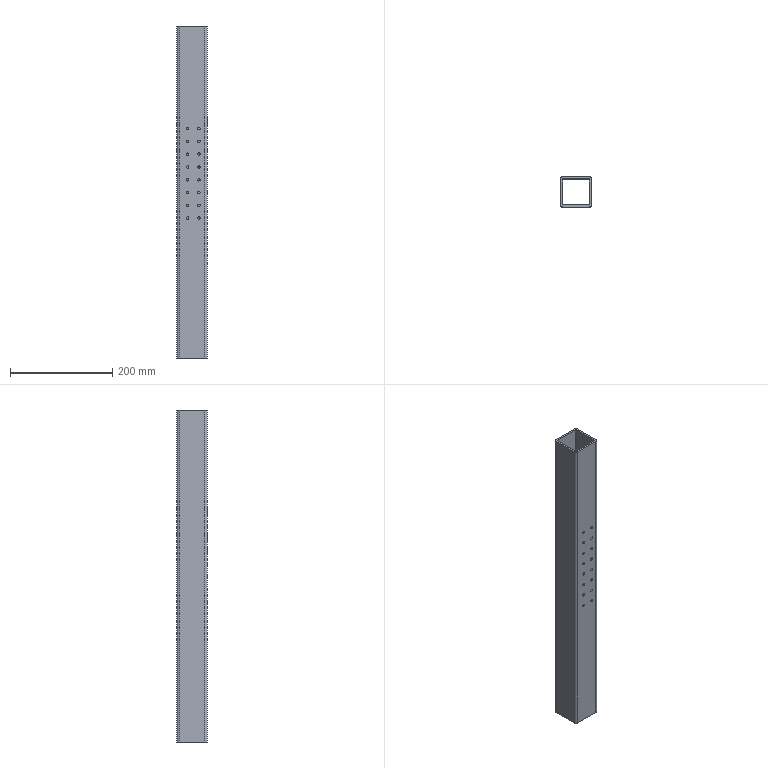Part | STEP file | 1 solid | 56 faces | box 60 x 60 x 650 mm | volume 567586 mm3 | cylinder 46 | plane 10 | commonest cylinder face diameters 5 x32 4.2 x6 2 x4 10 x4